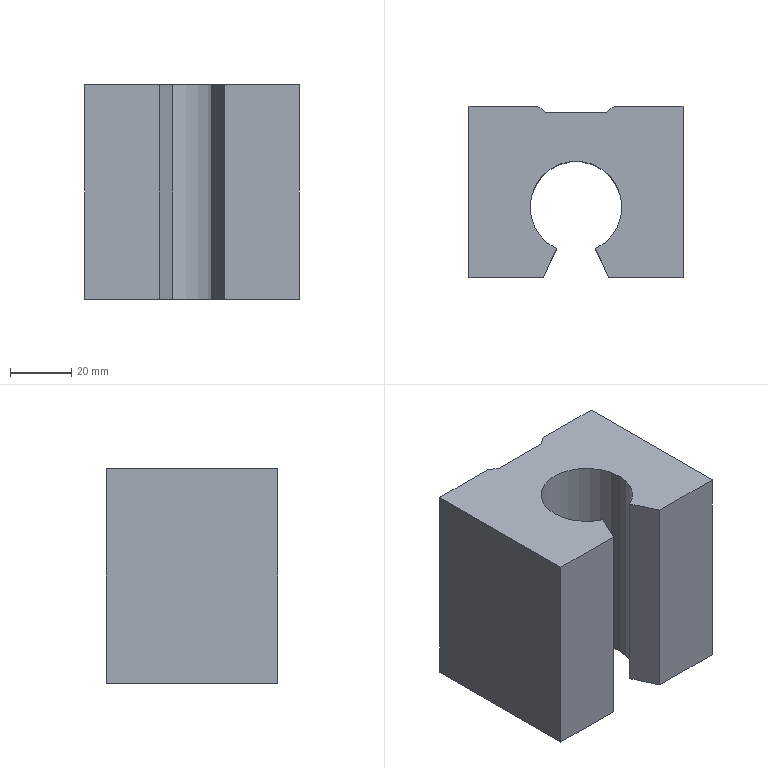Part | STEP file | 1 solid | 32 faces | box 70 x 56 x 70 mm | volume 208407 mm3 | plane 13 | cylinder 11 | cone 8 | commonest cylinder face diameters 6.8 x8 30 x3